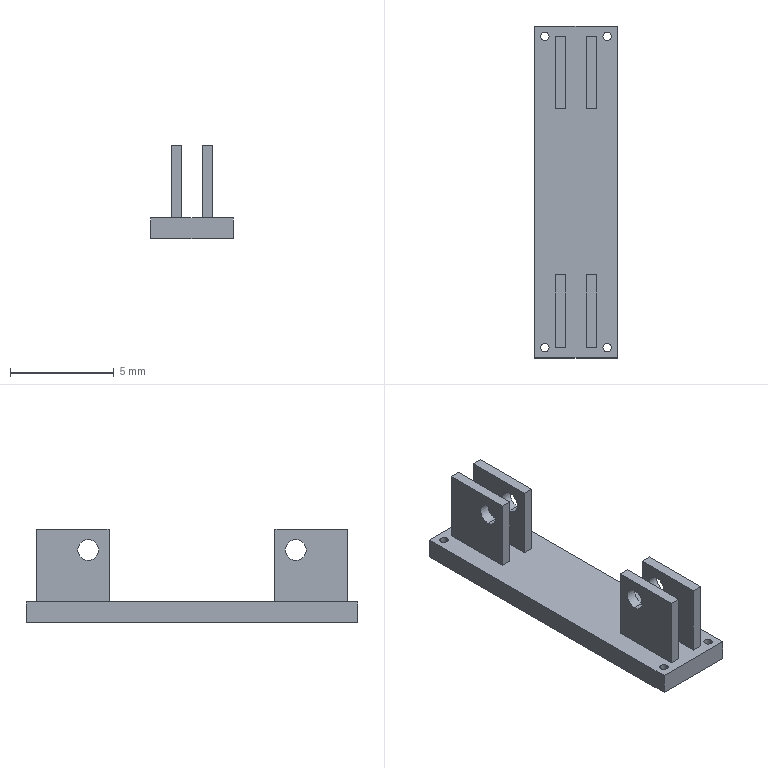Part | SolidWorks | features ICE 4, Extrusion 1 | 1 solid | 42 faces | box 4 x 16 x 4.5 mm | volume 86.427 mm3 | plane 26 | cylinder 16 | commonest cylinder face diameters 0.4 x8 1 x8
STEP:
#1=CARTESIAN_POINT('',(1.3,7.5,0.));
#2=VERTEX_POINT('',#1);
#3=CARTESIAN_POINT('',(1.7,7.5,0.));
#4=VERTEX_POINT('',#3);
#5=CARTESIAN_POINT('',(1.5,7.5,0.));
#6=DIRECTION('',(0.,0.,1.));
#7=DIRECTION('',(1.,0.,0.));
#8=AXIS2_PLACEMENT_3D('',#5,#6,#7);
#9=CIRCLE('',#8,0.2);
#10=EDGE_CURVE('',#2,#4,#9,.T.);
#11=ORIENTED_EDGE('',*,*,#10,.F.);
#12=CARTESIAN_POINT('',(1.3,7.5,1.));
#13=VERTEX_POINT('',#12);
#14=CARTESIAN_POINT('',(1.3,7.5,-3.5));
#15=DIRECTION('',(0.,0.,1.));
#16=VECTOR('',#15,1000.);
#17=LINE('',#14,#16);
#18=EDGE_CURVE('',#2,#13,#17,.T.);
#19=ORIENTED_EDGE('',*,*,#18,.T.);
#20=CARTESIAN_POINT('',(1.7,7.5,1.));
#21=VERTEX_POINT('',#20);
#22=CARTESIAN_POINT('',(1.5,7.5,1.));
#23=DIRECTION('',(0.,0.,1.));
#24=DIRECTION('',(1.,0.,0.));
#25=AXIS2_PLACEMENT_3D('',#22,#23,#24);
#26=CIRCLE('',#25,0.2);
#27=EDGE_CURVE('',#13,#21,#26,.T.);
#28=ORIENTED_EDGE('',*,*,#27,.T.);
#29=CARTESIAN_POINT('',(1.7,7.5,-3.5));
#30=DIRECTION('',(0.,0.,1.));
#31=VECTOR('',#30,1000.);
#32=LINE('',#29,#31);
#33=EDGE_CURVE('',#4,#21,#32,.T.);
#34=ORIENTED_EDGE('',*,*,#33,.F.);
#35=EDGE_LOOP('',(#11,#19,#28,#34));
#36=FACE_OUTER_BOUND('',#35,.T.);
#37=CARTESIAN_POINT('',(1.5,7.5,-3.5));
#38=DIRECTION('',(0.,0.,1.));
#39=DIRECTION('',(1.,0.,0.));
#40=AXIS2_PLACEMENT_3D('',#37,#38,#39);
#41=CYLINDRICAL_SURFACE('',#40,0.2);
#42=ADVANCED_FACE('',(#36),#41,.F.);
#43=CARTESIAN_POINT('',(1.3,-7.5,0.));
#44=VERTEX_POINT('',#43);
#45=CARTESIAN_POINT('',(1.7,-7.5,0.));
#46=VERTEX_POINT('',#45);
#47=CARTESIAN_POINT('',(1.5,-7.5,0.));
#48=DIRECTION('',(0.,0.,1.));
#49=DIRECTION('',(1.,0.,0.));
#50=AXIS2_PLACEMENT_3D('',#47,#48,#49);
#51=CIRCLE('',#50,0.2);
#52=EDGE_CURVE('',#44,#46,#51,.T.);
#53=ORIENTED_EDGE('',*,*,#52,.F.);
#54=CARTESIAN_POINT('',(1.3,-7.5,1.));
#55=VERTEX_POINT('',#54);
#56=CARTESIAN_POINT('',(1.3,-7.5,-3.5));
#57=DIRECTION('',(0.,0.,1.));
#58=VECTOR('',#57,1000.);
#59=LINE('',#56,#58);
#60=EDGE_CURVE('',#44,#55,#59,.T.);
#61=ORIENTED_EDGE('',*,*,#60,.T.);
#62=CARTESIAN_POINT('',(1.7,-7.5,1.));
#63=VERTEX_POINT('',#62);
#64=CARTESIAN_POINT('',(1.5,-7.5,1.));
#65=DIRECTION('',(0.,0.,1.));
#66=DIRECTION('',(1.,0.,0.));
#67=AXIS2_PLACEMENT_3D('',#64,#65,#66);
#68=CIRCLE('',#67,0.2);
#69=EDGE_CURVE('',#55,#63,#68,.T.);
#70=ORIENTED_EDGE('',*,*,#69,.T.);
#71=CARTESIAN_POINT('',(1.7,-7.5,-3.5));
#72=DIRECTION('',(0.,0.,1.));
#73=VECTOR('',#72,1000.);
#74=LINE('',#71,#73);
#75=EDGE_CURVE('',#46,#63,#74,.T.);
#76=ORIENTED_EDGE('',*,*,#75,.F.);
#77=EDGE_LOOP('',(#53,#61,#70,#76));
#78=FACE_OUTER_BOUND('',#77,.T.);
#79=CARTESIAN_POINT('',(1.5,-7.5,-3.5));
#80=DIRECTION('',(0.,0.,1.));
#81=DIRECTION('',(1.,0.,0.));
#82=AXIS2_PLACEMENT_3D('',#79,#80,#81);
#83=CYLINDRICAL_SURFACE('',#82,0.2);
#84=ADVANCED_FACE('',(#78),#83,.F.);
#85=CARTESIAN_POINT('',(-1.7,-7.5,0.));
#86=VERTEX_POINT('',#85);
#87=CARTESIAN_POINT('',(-1.3,-7.5,0.));
#88=VERTEX_POINT('',#87);
#89=CARTESIAN_POINT('',(-1.5,-7.5,0.));
#90=DIRECTION('',(0.,0.,1.));
#91=DIRECTION('',(1.,0.,0.));
#92=AXIS2_PLACEMENT_3D('',#89,#90,#91);
#93=CIRCLE('',#92,0.2);
#94=EDGE_CURVE('',#86,#88,#93,.T.);
#95=ORIENTED_EDGE('',*,*,#94,.F.);
#96=CARTESIAN_POINT('',(-1.7,-7.5,1.));
#97=VERTEX_POINT('',#96);
#98=CARTESIAN_POINT('',(-1.7,-7.5,-3.5));
#99=DIRECTION('',(0.,0.,1.));
#100=VECTOR('',#99,1000.);
#101=LINE('',#98,#100);
#102=EDGE_CURVE('',#86,#97,#101,.T.);
#103=ORIENTED_EDGE('',*,*,#102,.T.);
#104=CARTESIAN_POINT('',(-1.3,-7.5,1.));
#105=VERTEX_POINT('',#104);
#106=CARTESIAN_POINT('',(-1.5,-7.5,1.));
#107=DIRECTION('',(0.,0.,1.));
#108=DIRECTION('',(1.,0.,0.));
#109=AXIS2_PLACEMENT_3D('',#106,#107,#108);
#110=CIRCLE('',#109,0.2);
#111=EDGE_CURVE('',#97,#105,#110,.T.);
#112=ORIENTED_EDGE('',*,*,#111,.T.);
#113=CARTESIAN_POINT('',(-1.3,-7.5,-3.5));
#114=DIRECTION('',(0.,0.,1.));
#115=VECTOR('',#114,1000.);
#116=LINE('',#113,#115);
#117=EDGE_CURVE('',#88,#105,#116,.T.);
#118=ORIENTED_EDGE('',*,*,#117,.F.);
#119=EDGE_LOOP('',(#95,#103,#112,#118));
#120=FACE_OUTER_BOUND('',#119,.T.);
#121=CARTESIAN_POINT('',(-1.5,-7.5,-3.5));
#122=DIRECTION('',(0.,0.,1.));
#123=DIRECTION('',(1.,0.,0.));
#124=AXIS2_PLACEMENT_3D('',#121,#122,#123);
#125=CYLINDRICAL_SURFACE('',#124,0.2);
#126=ADVANCED_FACE('',(#120),#125,.F.);
#127=CARTESIAN_POINT('',(-1.7,7.5,0.));
#128=VERTEX_POINT('',#127);
#129=CARTESIAN_POINT('',(-1.3,7.5,0.));
#130=VERTEX_POINT('',#129);
#131=CARTESIAN_POINT('',(-1.5,7.5,0.));
#132=DIRECTION('',(0.,0.,1.));
#133=DIRECTION('',(1.,0.,0.));
#134=AXIS2_PLACEMENT_3D('',#131,#132,#133);
#135=CIRCLE('',#134,0.2);
#136=EDGE_CURVE('',#128,#130,#135,.T.);
#137=ORIENTED_EDGE('',*,*,#136,.F.);
#138=CARTESIAN_POINT('',(-1.7,7.5,1.));
#139=VERTEX_POINT('',#138);
#140=CARTESIAN_POINT('',(-1.7,7.5,-3.5));
#141=DIRECTION('',(0.,0.,1.));
#142=VECTOR('',#141,1000.);
#143=LINE('',#140,#142);
#144=EDGE_CURVE('',#128,#139,#143,.T.);
#145=ORIENTED_EDGE('',*,*,#144,.T.);
#146=CARTESIAN_POINT('',(-1.3,7.5,1.));
#147=VERTEX_POINT('',#146);
#148=CARTESIAN_POINT('',(-1.5,7.5,1.));
#149=DIRECTION('',(0.,0.,1.));
#150=DIRECTION('',(1.,0.,0.));
#151=AXIS2_PLACEMENT_3D('',#148,#149,#150);
#152=CIRCLE('',#151,0.2);
#153=EDGE_CURVE('',#139,#147,#152,.T.);
#154=ORIENTED_EDGE('',*,*,#153,.T.);
#155=CARTESIAN_POINT('',(-1.3,7.5,-3.5));
#156=DIRECTION('',(0.,0.,1.));
#157=VECTOR('',#156,1000.);
#158=LINE('',#155,#157);
#159=EDGE_CURVE('',#130,#147,#158,.T.);
#160=ORIENTED_EDGE('',*,*,#159,.F.);
#161=EDGE_LOOP('',(#137,#145,#154,#160));
#162=FACE_OUTER_BOUND('',#161,.T.);
#163=CARTESIAN_POINT('',(-1.5,7.5,-3.5));
#164=DIRECTION('',(0.,0.,1.));
#165=DIRECTION('',(1.,0.,0.));
#166=AXIS2_PLACEMENT_3D('',#163,#164,#165);
#167=CYLINDRICAL_SURFACE('',#166,0.2);
#168=ADVANCED_FACE('',(#162),#167,.F.);
#169=CARTESIAN_POINT('',(1.,5.,3.));
#170=VERTEX_POINT('',#169);
#171=CARTESIAN_POINT('',(1.,5.,4.));
#172=VERTEX_POINT('',#171);
#173=CARTESIAN_POINT('',(1.,5.,3.5));
#174=DIRECTION('',(-1.,0.,0.));
#175=DIRECTION('',(0.,0.,1.));
#176=AXIS2_PLACEMENT_3D('',#173,#174,#175);
#177=CIRCLE('',#176,0.5);
#178=EDGE_CURVE('',#170,#172,#177,.T.);
#179=ORIENTED_EDGE('',*,*,#178,.F.);
#180=CARTESIAN_POINT('',(0.5,5.,3.));
#181=VERTEX_POINT('',#180);
#182=CARTESIAN_POINT('',(3.5,5.,3.));
#183=DIRECTION('',(-1.,0.,0.));
#184=VECTOR('',#183,1000.);
#185=LINE('',#182,#184);
#186=EDGE_CURVE('',#170,#181,#185,.T.);
#187=ORIENTED_EDGE('',*,*,#186,.T.);
#188=CARTESIAN_POINT('',(0.5,5.,4.));
#189=VERTEX_POINT('',#188);
#190=CARTESIAN_POINT('',(0.5,5.,3.5));
#191=DIRECTION('',(1.,0.,0.));
#192=DIRECTION('',(0.,0.,-1.));
#193=AXIS2_PLACEMENT_3D('',#190,#191,#192);
#194=CIRCLE('',#193,0.5);
#195=EDGE_CURVE('',#189,#181,#194,.T.);
#196=ORIENTED_EDGE('',*,*,#195,.F.);
#197=CARTESIAN_POINT('',(3.5,5.,4.));
#198=DIRECTION('',(-1.,0.,0.));
#199=VECTOR('',#198,1000.);
#200=LINE('',#197,#199);
#201=EDGE_CURVE('',#172,#189,#200,.T.);
#202=ORIENTED_EDGE('',*,*,#201,.F.);
#203=EDGE_LOOP('',(#179,#187,#196,#202));
#204=FACE_OUTER_BOUND('',#203,.T.);
#205=CARTESIAN_POINT('',(3.5,5.,3.5));
#206=DIRECTION('',(-1.,0.,0.));
#207=DIRECTION('',(0.,0.,1.));
#208=AXIS2_PLACEMENT_3D('',#205,#206,#207);
#209=CYLINDRICAL_SURFACE('',#208,0.5);
#210=ADVANCED_FACE('',(#204),#209,.F.);
#211=CARTESIAN_POINT('',(1.,-5.,3.));
#212=VERTEX_POINT('',#211);
#213=CARTESIAN_POINT('',(1.,-5.,4.));
#214=VERTEX_POINT('',#213);
#215=CARTESIAN_POINT('',(1.,-5.,3.5));
#216=DIRECTION('',(-1.,0.,0.));
#217=DIRECTION('',(0.,0.,1.));
#218=AXIS2_PLACEMENT_3D('',#215,#216,#217);
#219=CIRCLE('',#218,0.5);
#220=EDGE_CURVE('',#212,#214,#219,.T.);
#221=ORIENTED_EDGE('',*,*,#220,.F.);
#222=CARTESIAN_POINT('',(0.5,-5.,3.));
#223=VERTEX_POINT('',#222);
#224=CARTESIAN_POINT('',(3.5,-5.,3.));
#225=DIRECTION('',(-1.,0.,0.));
#226=VECTOR('',#225,1000.);
#227=LINE('',#224,#226);
#228=EDGE_CURVE('',#212,#223,#227,.T.);
#229=ORIENTED_EDGE('',*,*,#228,.T.);
#230=CARTESIAN_POINT('',(0.5,-5.,4.));
#231=VERTEX_POINT('',#230);
#232=CARTESIAN_POINT('',(0.5,-5.,3.5));
#233=DIRECTION('',(1.,0.,0.));
#234=DIRECTION('',(0.,0.,-1.));
#235=AXIS2_PLACEMENT_3D('',#232,#233,#234);
#236=CIRCLE('',#235,0.5);
#237=EDGE_CURVE('',#231,#223,#236,.T.);
#238=ORIENTED_EDGE('',*,*,#237,.F.);
#239=CARTESIAN_POINT('',(3.5,-5.,4.));
#240=DIRECTION('',(-1.,0.,0.));
#241=VECTOR('',#240,1000.);
#242=LINE('',#239,#241);
#243=EDGE_CURVE('',#214,#231,#242,.T.);
#244=ORIENTED_EDGE('',*,*,#243,.F.);
#245=EDGE_LOOP('',(#221,#229,#238,#244));
#246=FACE_OUTER_BOUND('',#245,.T.);
#247=CARTESIAN_POINT('',(3.5,-5.,3.5));
#248=DIRECTION('',(-1.,0.,0.));
#249=DIRECTION('',(0.,0.,1.));
#250=AXIS2_PLACEMENT_3D('',#247,#248,#249);
#251=CYLINDRICAL_SURFACE('',#250,0.5);
#252=ADVANCED_FACE('',(#246),#251,.F.);
#253=CARTESIAN_POINT('',(-0.5,5.,3.));
#254=VERTEX_POINT('',#253);
#255=CARTESIAN_POINT('',(-0.5,5.,4.));
#256=VERTEX_POINT('',#255);
#257=CARTESIAN_POINT('',(-0.5,5.,3.5));
#258=DIRECTION('',(-1.,0.,0.));
#259=DIRECTION('',(0.,0.,1.));
#260=AXIS2_PLACEMENT_3D('',#257,#258,#259);
#261=CIRCLE('',#260,0.5);
#262=EDGE_CURVE('',#254,#256,#261,.T.);
#263=ORIENTED_EDGE('',*,*,#262,.F.);
#264=CARTESIAN_POINT('',(-1.,5.,3.));
#265=VERTEX_POINT('',#264);
#266=CARTESIAN_POINT('',(3.5,5.,3.));
#267=DIRECTION('',(-1.,0.,0.));
#268=VECTOR('',#267,1000.);
#269=LINE('',#266,#268);
#270=EDGE_CURVE('',#254,#265,#269,.T.);
#271=ORIENTED_EDGE('',*,*,#270,.T.);
#272=CARTESIAN_POINT('',(-1.,5.,4.));
#273=VERTEX_POINT('',#272);
#274=CARTESIAN_POINT('',(-1.,5.,3.5));
#275=DIRECTION('',(-1.,0.,0.));
#276=DIRECTION('',(0.,0.,1.));
#277=AXIS2_PLACEMENT_3D('',#274,#275,#276);
#278=CIRCLE('',#277,0.5);
#279=EDGE_CURVE('',#265,#273,#278,.T.);
#280=ORIENTED_EDGE('',*,*,#279,.T.);
#281=CARTESIAN_POINT('',(3.5,5.,4.));
#282=DIRECTION('',(-1.,0.,0.));
#283=VECTOR('',#282,1000.);
#284=LINE('',#281,#283);
#285=EDGE_CURVE('',#256,#273,#284,.T.);
#286=ORIENTED_EDGE('',*,*,#285,.F.);
#287=EDGE_LOOP('',(#263,#271,#280,#286));
#288=FACE_OUTER_BOUND('',#287,.T.);
#289=CARTESIAN_POINT('',(3.5,5.,3.5));
#290=DIRECTION('',(-1.,0.,0.));
#291=DIRECTION('',(0.,0.,1.));
#292=AXIS2_PLACEMENT_3D('',#289,#290,#291);
#293=CYLINDRICAL_SURFACE('',#292,0.5);
#294=ADVANCED_FACE('',(#288),#293,.F.);
#295=CARTESIAN_POINT('',(-0.5,-5.,3.));
#296=VERTEX_POINT('',#295);
#297=CARTESIAN_POINT('',(-0.5,-5.,4.));
#298=VERTEX_POINT('',#297);
#299=CARTESIAN_POINT('',(-0.5,-5.,3.5));
#300=DIRECTION('',(-1.,0.,0.));
#301=DIRECTION('',(0.,0.,1.));
#302=AXIS2_PLACEMENT_3D('',#299,#300,#301);
#303=CIRCLE('',#302,0.5);
#304=EDGE_CURVE('',#296,#298,#303,.T.);
#305=ORIENTED_EDGE('',*,*,#304,.F.);
#306=CARTESIAN_POINT('',(-1.,-5.,3.));
#307=VERTEX_POINT('',#306);
#308=CARTESIAN_POINT('',(3.5,-5.,3.));
#309=DIRECTION('',(-1.,0.,0.));
#310=VECTOR('',#309,1000.);
#311=LINE('',#308,#310);
#312=EDGE_CURVE('',#296,#307,#311,.T.);
#313=ORIENTED_EDGE('',*,*,#312,.T.);
#314=CARTESIAN_POINT('',(-1.,-5.,4.));
#315=VERTEX_POINT('',#314);
#316=CARTESIAN_POINT('',(-1.,-5.,3.5));
#317=DIRECTION('',(-1.,0.,0.));
#318=DIRECTION('',(0.,0.,1.));
#319=AXIS2_PLACEMENT_3D('',#316,#317,#318);
#320=CIRCLE('',#319,0.5);
#321=EDGE_CURVE('',#307,#315,#320,.T.);
#322=ORIENTED_EDGE('',*,*,#321,.T.);
#323=CARTESIAN_POINT('',(3.5,-5.,4.));
#324=DIRECTION('',(-1.,0.,0.));
#325=VECTOR('',#324,1000.);
#326=LINE('',#323,#325);
#327=EDGE_CURVE('',#298,#315,#326,.T.);
#328=ORIENTED_EDGE('',*,*,#327,.F.);
#329=EDGE_LOOP('',(#305,#313,#322,#328));
#330=FACE_OUTER_BOUND('',#329,.T.);
#331=CARTESIAN_POINT('',(3.5,-5.,3.5));
#332=DIRECTION('',(-1.,0.,0.));
#333=DIRECTION('',(0.,0.,1.));
#334=AXIS2_PLACEMENT_3D('',#331,#332,#333);
#335=CYLINDRICAL_SURFACE('',#334,0.5);
#336=ADVANCED_FACE('',(#330),#335,.F.);
#337=CARTESIAN_POINT('',(1.,-5.,3.5));
#338=DIRECTION('',(-1.,0.,0.));
#339=DIRECTION('',(0.,0.,1.));
#340=AXIS2_PLACEMENT_3D('',#337,#338,#339);
#341=CIRCLE('',#340,0.5);
#342=EDGE_CURVE('',#214,#212,#341,.T.);
#343=ORIENTED_EDGE('',*,*,#342,.T.);
#344=ORIENTED_EDGE('',*,*,#220,.T.);
#345=EDGE_LOOP('',(#343,#344));
#346=FACE_BOUND('',#345,.T.);
#347=CARTESIAN_POINT('',(1.,-7.5,1.));
#348=VERTEX_POINT('',#347);
#349=CARTESIAN_POINT('',(1.,-4.,1.));
#350=VERTEX_POINT('',#349);
#351=CARTESIAN_POINT('',(1.,-7.5,1.));
#352=DIRECTION('',(0.,1.,0.));
#353=VECTOR('',#352,1000.);
#354=LINE('',#351,#353);
#355=EDGE_CURVE('',#348,#350,#354,.T.);
#356=ORIENTED_EDGE('',*,*,#355,.T.);
#357=CARTESIAN_POINT('',(1.,-4.,4.5));
#358=VERTEX_POINT('',#357);
#359=CARTESIAN_POINT('',(1.,-4.,4.5));
#360=DIRECTION('',(0.,0.,1.));
#361=VECTOR('',#360,1000.);
#362=LINE('',#359,#361);
#363=EDGE_CURVE('',#350,#358,#362,.T.);
#364=ORIENTED_EDGE('',*,*,#363,.T.);
#365=CARTESIAN_POINT('',(1.,-7.5,4.5));
#366=VERTEX_POINT('',#365);
#367=CARTESIAN_POINT('',(1.,-7.5,4.5));
#368=DIRECTION('',(0.,1.,0.));
#369=VECTOR('',#368,1000.);
#370=LINE('',#367,#369);
#371=EDGE_CURVE('',#366,#358,#370,.T.);
#372=ORIENTED_EDGE('',*,*,#371,.F.);
#373=CARTESIAN_POINT('',(1.,-7.5,4.5));
#374=DIRECTION('',(0.,0.,-1.));
#375=VECTOR('',#374,1000.);
#376=LINE('',#373,#375);
#377=EDGE_CURVE('',#366,#348,#376,.T.);
#378=ORIENTED_EDGE('',*,*,#377,.T.);
#379=EDGE_LOOP('',(#356,#364,#372,#378));
#380=FACE_OUTER_BOUND('',#379,.T.);
#381=CARTESIAN_POINT('',(1.,-7.5,4.5));
#382=DIRECTION('',(-1.,0.,0.));
#383=DIRECTION('',(0.,0.,1.));
#384=AXIS2_PLACEMENT_3D('',#381,#382,#383);
#385=PLANE('',#384);
#386=ADVANCED_FACE('',(#346,#380),#385,.F.);
#387=ORIENTED_EDGE('',*,*,#237,.T.);
#388=CARTESIAN_POINT('',(0.5,-5.,3.5));
#389=DIRECTION('',(1.,0.,0.));
#390=DIRECTION('',(0.,0.,-1.));
#391=AXIS2_PLACEMENT_3D('',#388,#389,#390);
#392=CIRCLE('',#391,0.5);
#393=EDGE_CURVE('',#223,#231,#392,.T.);
#394=ORIENTED_EDGE('',*,*,#393,.T.);
#395=EDGE_LOOP('',(#387,#394));
#396=FACE_BOUND('',#395,.T.);
#397=CARTESIAN_POINT('',(0.5,-4.,4.5));
#398=VERTEX_POINT('',#397);
#399=CARTESIAN_POINT('',(0.5,-7.5,4.5));
#400=VERTEX_POINT('',#399);
#401=CARTESIAN_POINT('',(0.5,-7.5,4.5));
#402=DIRECTION('',(0.,-1.,0.));
#403=VECTOR('',#402,1000.);
#404=LINE('',#401,#403);
#405=EDGE_CURVE('',#398,#400,#404,.T.);
#406=ORIENTED_EDGE('',*,*,#405,.F.);
#407=CARTESIAN_POINT('',(0.5,-4.,1.));
#408=VERTEX_POINT('',#407);
#409=CARTESIAN_POINT('',(0.5,-4.,4.5));
#410=DIRECTION('',(0.,0.,-1.));
#411=VECTOR('',#410,1000.);
#412=LINE('',#409,#411);
#413=EDGE_CURVE('',#398,#408,#412,.T.);
#414=ORIENTED_EDGE('',*,*,#413,.T.);
#415=CARTESIAN_POINT('',(0.5,-7.5,1.));
#416=VERTEX_POINT('',#415);
#417=CARTESIAN_POINT('',(0.5,-7.5,1.));
#418=DIRECTION('',(0.,-1.,0.));
#419=VECTOR('',#418,1000.);
#420=LINE('',#417,#419);
#421=EDGE_CURVE('',#408,#416,#420,.T.);
#422=ORIENTED_EDGE('',*,*,#421,.T.);
#423=CARTESIAN_POINT('',(0.5,-7.5,4.5));
#424=DIRECTION('',(0.,0.,-1.));
#425=VECTOR('',#424,1000.);
#426=LINE('',#423,#425);
#427=EDGE_CURVE('',#400,#416,#426,.T.);
#428=ORIENTED_EDGE('',*,*,#427,.F.);
#429=EDGE_LOOP('',(#406,#414,#422,#428));
#430=FACE_OUTER_BOUND('',#429,.T.);
#431=CARTESIAN_POINT('',(0.5,-7.5,4.5));
#432=DIRECTION('',(1.,0.,0.));
#433=DIRECTION('',(0.,0.,-1.));
#434=AXIS2_PLACEMENT_3D('',#431,#432,#433);
#435=PLANE('',#434);
#436=ADVANCED_FACE('',(#396,#430),#435,.F.);
#437=ORIENTED_EDGE('',*,*,#371,.T.);
#438=CARTESIAN_POINT('',(-4.096,-4.,4.5));
#439=DIRECTION('',(1.,0.,0.));
#440=VECTOR('',#439,1000.);
#441=LINE('',#438,#440);
#442=EDGE_CURVE('',#398,#358,#441,.T.);
#443=ORIENTED_EDGE('',*,*,#442,.F.);
#444=ORIENTED_EDGE('',*,*,#405,.T.);
#445=CARTESIAN_POINT('',(0.5,-7.5,4.5));
#446=DIRECTION('',(1.,0.,0.));
#447=VECTOR('',#446,1000.);
#448=LINE('',#445,#447);
#449=EDGE_CURVE('',#400,#366,#448,.T.);
#450=ORIENTED_EDGE('',*,*,#449,.T.);
#451=EDGE_LOOP('',(#437,#443,#444,#450));
#452=FACE_OUTER_BOUND('',#451,.T.);
#453=CARTESIAN_POINT('',(0.,0.,4.5));
#454=DIRECTION('',(0.,0.,-1.));
#455=DIRECTION('',(-1.,0.,0.));
#456=AXIS2_PLACEMENT_3D('',#453,#454,#455);
#457=PLANE('',#456);
#458=ADVANCED_FACE('',(#452),#457,.F.);
#459=CARTESIAN_POINT('',(-1.,-5.,3.5));
#460=DIRECTION('',(-1.,0.,0.));
#461=DIRECTION('',(0.,0.,1.));
#462=AXIS2_PLACEMENT_3D('',#459,#460,#461);
#463=CIRCLE('',#462,0.5);
#464=EDGE_CURVE('',#315,#307,#463,.T.);
#465=ORIENTED_EDGE('',*,*,#464,.F.);
#466=ORIENTED_EDGE('',*,*,#321,.F.);
#467=EDGE_LOOP('',(#465,#466));
#468=FACE_BOUND('',#467,.T.);
#469=CARTESIAN_POINT('',(-1.,-4.,4.5));
#470=VERTEX_POINT('',#469);
#471=CARTESIAN_POINT('',(-1.,-7.5,4.5));
#472=VERTEX_POINT('',#471);
#473=CARTESIAN_POINT('',(-1.,-7.5,4.5));
#474=DIRECTION('',(0.,-1.,0.));
#475=VECTOR('',#474,1000.);
#476=LINE('',#473,#475);
#477=EDGE_CURVE('',#470,#472,#476,.T.);
#478=ORIENTED_EDGE('',*,*,#477,.F.);
#479=CARTESIAN_POINT('',(-1.,-4.,1.));
#480=VERTEX_POINT('',#479);
#481=CARTESIAN_POINT('',(-1.,-4.,4.5));
#482=DIRECTION('',(0.,0.,-1.));
#483=VECTOR('',#482,1000.);
#484=LINE('',#481,#483);
#485=EDGE_CURVE('',#470,#480,#484,.T.);
#486=ORIENTED_EDGE('',*,*,#485,.T.);
#487=CARTESIAN_POINT('',(-1.,-7.5,1.));
#488=VERTEX_POINT('',#487);
#489=CARTESIAN_POINT('',(-1.,-7.5,1.));
#490=DIRECTION('',(0.,-1.,0.));
#491=VECTOR('',#490,1000.);
#492=LINE('',#489,#491);
#493=EDGE_CURVE('',#480,#488,#492,.T.);
#494=ORIENTED_EDGE('',*,*,#493,.T.);
#495=CARTESIAN_POINT('',(-1.,-7.5,4.5));
#496=DIRECTION('',(0.,0.,-1.));
#497=VECTOR('',#496,1000.);
#498=LINE('',#495,#497);
#499=EDGE_CURVE('',#472,#488,#498,.T.);
#500=ORIENTED_EDGE('',*,*,#499,.F.);
#501=EDGE_LOOP('',(#478,#486,#494,#500));
#502=FACE_OUTER_BOUND('',#501,.T.);
#503=CARTESIAN_POINT('',(-1.,-7.5,4.5));
#504=DIRECTION('',(1.,0.,0.));
#505=DIRECTION('',(0.,1.,0.));
#506=AXIS2_PLACEMENT_3D('',#503,#504,#505);
#507=PLANE('',#506);
#508=ADVANCED_FACE('',(#468,#502),#507,.F.);
#509=CARTESIAN_POINT('',(-0.5,-5.,3.5));
#510=DIRECTION('',(-1.,0.,0.));
#511=DIRECTION('',(0.,0.,1.));
#512=AXIS2_PLACEMENT_3D('',#509,#510,#511);
#513=CIRCLE('',#512,0.5);
#514=EDGE_CURVE('',#298,#296,#513,.T.);
#515=ORIENTED_EDGE('',*,*,#514,.T.);
#516=ORIENTED_EDGE('',*,*,#304,.T.);
#517=EDGE_LOOP('',(#515,#516));
#518=FACE_BOUND('',#517,.T.);
#519=CARTESIAN_POINT('',(-0.5,-7.5,1.));
#520=VERTEX_POINT('',#519);
#521=CARTESIAN_POINT('',(-0.5,-4.,1.));
#522=VERTEX_POINT('',#521);
#523=CARTESIAN_POINT('',(-0.5,-7.5,1.));
#524=DIRECTION('',(0.,1.,0.));
#525=VECTOR('',#524,1000.);
#526=LINE('',#523,#525);
#527=EDGE_CURVE('',#520,#522,#526,.T.);
#528=ORIENTED_EDGE('',*,*,#527,.T.);
#529=CARTESIAN_POINT('',(-0.5,-4.,4.5));
#530=VERTEX_POINT('',#529);
#531=CARTESIAN_POINT('',(-0.5,-4.,4.5));
#532=DIRECTION('',(0.,0.,1.));
#533=VECTOR('',#532,1000.);
#534=LINE('',#531,#533);
#535=EDGE_CURVE('',#522,#530,#534,.T.);
#536=ORIENTED_EDGE('',*,*,#535,.T.);
#537=CARTESIAN_POINT('',(-0.5,-7.5,4.5));
#538=VERTEX_POINT('',#537);
#539=CARTESIAN_POINT('',(-0.5,-7.5,4.5));
#540=DIRECTION('',(0.,1.,0.));
#541=VECTOR('',#540,1000.);
#542=LINE('',#539,#541);
#543=EDGE_CURVE('',#538,#530,#542,.T.);
#544=ORIENTED_EDGE('',*,*,#543,.F.);
#545=CARTESIAN_POINT('',(-0.5,-7.5,4.5));
#546=DIRECTION('',(0.,0.,-1.));
#547=VECTOR('',#546,1000.);
#548=LINE('',#545,#547);
#549=EDGE_CURVE('',#538,#520,#548,.T.);
#550=ORIENTED_EDGE('',*,*,#549,.T.);
#551=EDGE_LOOP('',(#528,#536,#544,#550));
#552=FACE_OUTER_BOUND('',#551,.T.);
#553=CARTESIAN_POINT('',(-0.5,-7.5,4.5));
#554=DIRECTION('',(-1.,0.,0.));
#555=DIRECTION('',(0.,0.,1.));
#556=AXIS2_PLACEMENT_3D('',#553,#554,#555);
#557=PLANE('',#556);
#558=ADVANCED_FACE('',(#518,#552),#557,.F.);
#559=CARTESIAN_POINT('',(0.,-4.,4.5));
#560=DIRECTION('',(1.,0.,0.));
#561=VECTOR('',#560,1000.);
#562=LINE('',#559,#561);
#563=EDGE_CURVE('',#470,#530,#562,.T.);
#564=ORIENTED_EDGE('',*,*,#563,.F.);
#565=ORIENTED_EDGE('',*,*,#477,.T.);
#566=CARTESIAN_POINT('',(-0.5,-7.5,4.5));
#567=DIRECTION('',(1.,0.,0.));
#568=VECTOR('',#567,1000.);
#569=LINE('',#566,#568);
#570=EDGE_CURVE('',#472,#538,#569,.T.);
#571=ORIENTED_EDGE('',*,*,#570,.T.);
#572=ORIENTED_EDGE('',*,*,#543,.T.);
#573=EDGE_LOOP('',(#564,#565,#571,#572));
#574=FACE_OUTER_BOUND('',#573,.T.);
#575=CARTESIAN_POINT('',(0.,0.,4.5));
#576=DIRECTION('',(0.,0.,1.));
#577=DIRECTION('',(1.,0.,0.));
#578=AXIS2_PLACEMENT_3D('',#575,#576,#577);
#579=PLANE('',#578);
#580=ADVANCED_FACE('',(#574),#579,.T.);
#581=ORIENTED_EDGE('',*,*,#493,.F.);
#582=CARTESIAN_POINT('',(-4.096,-4.,1.));
#583=DIRECTION('',(-1.,0.,0.));
#584=VECTOR('',#583,1000.);
#585=LINE('',#582,#584);
#586=EDGE_CURVE('',#522,#480,#585,.T.);
#587=ORIENTED_EDGE('',*,*,#586,.F.);
#588=ORIENTED_EDGE('',*,*,#527,.F.);
#589=CARTESIAN_POINT('',(-0.5,-7.5,1.));
#590=DIRECTION('',(1.,0.,0.));
#591=VECTOR('',#590,1000.);
#592=LINE('',#589,#591);
#593=EDGE_CURVE('',#488,#520,#592,.T.);
#594=ORIENTED_EDGE('',*,*,#593,.F.);
#595=EDGE_LOOP('',(#581,#587,#588,#594));
#596=FACE_BOUND('',#595,.T.);
#597=ORIENTED_EDGE('',*,*,#421,.F.);
#598=CARTESIAN_POINT('',(-4.096,-4.,1.));
#599=DIRECTION('',(-1.,0.,0.));
#600=VECTOR('',#599,1000.);
#601=LINE('',#598,#600);
#602=EDGE_CURVE('',#350,#408,#601,.T.);
#603=ORIENTED_EDGE('',*,*,#602,.F.);
#604=ORIENTED_EDGE('',*,*,#355,.F.);
#605=CARTESIAN_POINT('',(0.5,-7.5,1.));
#606=DIRECTION('',(1.,0.,0.));
#607=VECTOR('',#606,1000.);
#608=LINE('',#605,#607);
#609=EDGE_CURVE('',#416,#348,#608,.T.);
#610=ORIENTED_EDGE('',*,*,#609,.F.);
#611=EDGE_LOOP('',(#597,#603,#604,#610));
#612=FACE_BOUND('',#611,.T.);
#613=CARTESIAN_POINT('',(1.,4.,1.));
#614=VERTEX_POINT('',#613);
#615=CARTESIAN_POINT('',(1.,7.5,1.));
#616=VERTEX_POINT('',#615);
#617=CARTESIAN_POINT('',(1.,-7.5,1.));
#618=DIRECTION('',(0.,1.,0.));
#619=VECTOR('',#618,1000.);
#620=LINE('',#617,#619);
#621=EDGE_CURVE('',#614,#616,#620,.T.);
#622=ORIENTED_EDGE('',*,*,#621,.F.);
#623=CARTESIAN_POINT('',(0.5,4.,1.));
#624=VERTEX_POINT('',#623);
#625=CARTESIAN_POINT('',(-4.096,4.,1.));
#626=DIRECTION('',(1.,0.,0.));
#627=VECTOR('',#626,1000.);
#628=LINE('',#625,#627);
#629=EDGE_CURVE('',#624,#614,#628,.T.);
#630=ORIENTED_EDGE('',*,*,#629,.F.);
#631=CARTESIAN_POINT('',(0.5,7.5,1.));
#632=VERTEX_POINT('',#631);
#633=CARTESIAN_POINT('',(0.5,-7.5,1.));
#634=DIRECTION('',(0.,-1.,0.));
#635=VECTOR('',#634,1000.);
#636=LINE('',#633,#635);
#637=EDGE_CURVE('',#632,#624,#636,.T.);
#638=ORIENTED_EDGE('',*,*,#637,.F.);
#639=CARTESIAN_POINT('',(0.5,7.5,1.));
#640=DIRECTION('',(-1.,0.,0.));
#641=VECTOR('',#640,1000.);
#642=LINE('',#639,#641);
#643=EDGE_CURVE('',#616,#632,#642,.T.);
#644=ORIENTED_EDGE('',*,*,#643,.F.);
#645=EDGE_LOOP('',(#622,#630,#638,#644));
#646=FACE_BOUND('',#645,.T.);
#647=CARTESIAN_POINT('',(-0.5,4.,1.));
#648=VERTEX_POINT('',#647);
#649=CARTESIAN_POINT('',(-0.5,7.5,1.));
#650=VERTEX_POINT('',#649);
#651=CARTESIAN_POINT('',(-0.5,-7.5,1.));
#652=DIRECTION('',(0.,1.,0.));
#653=VECTOR('',#652,1000.);
#654=LINE('',#651,#653);
#655=EDGE_CURVE('',#648,#650,#654,.T.);
#656=ORIENTED_EDGE('',*,*,#655,.F.);
#657=CARTESIAN_POINT('',(-1.,4.,1.));
#658=VERTEX_POINT('',#657);
#659=CARTESIAN_POINT('',(-4.096,4.,1.));
#660=DIRECTION('',(1.,0.,0.));
#661=VECTOR('',#660,1000.);
#662=LINE('',#659,#661);
#663=EDGE_CURVE('',#658,#648,#662,.T.);
#664=ORIENTED_EDGE('',*,*,#663,.F.);
#665=CARTESIAN_POINT('',(-1.,7.5,1.));
#666=VERTEX_POINT('',#665);
#667=CARTESIAN_POINT('',(-1.,-7.5,1.));
#668=DIRECTION('',(0.,-1.,0.));
#669=VECTOR('',#668,1000.);
#670=LINE('',#667,#669);
#671=EDGE_CURVE('',#666,#658,#670,.T.);
#672=ORIENTED_EDGE('',*,*,#671,.F.);
#673=CARTESIAN_POINT('',(-0.5,7.5,1.));
#674=DIRECTION('',(-1.,0.,0.));
#675=VECTOR('',#674,1000.);
#676=LINE('',#673,#675);
#677=EDGE_CURVE('',#650,#666,#676,.T.);
#678=ORIENTED_EDGE('',*,*,#677,.F.);
#679=EDGE_LOOP('',(#656,#664,#672,#678));
#680=FACE_BOUND('',#679,.T.);
#681=CARTESIAN_POINT('',(2.,-8.,1.));
#682=VERTEX_POINT('',#681);
#683=CARTESIAN_POINT('',(2.,8.,1.));
#684=VERTEX_POINT('',#683);
#685=CARTESIAN_POINT('',(2.,-8.,1.));
#686=DIRECTION('',(0.,1.,0.));
#687=VECTOR('',#686,1000.);
#688=LINE('',#685,#687);
#689=EDGE_CURVE('',#682,#684,#688,.T.);
#690=ORIENTED_EDGE('',*,*,#689,.T.);
#691=CARTESIAN_POINT('',(-2.,8.,1.));
#692=VERTEX_POINT('',#691);
#693=CARTESIAN_POINT('',(2.,8.,1.));
#694=DIRECTION('',(-1.,0.,0.));
#695=VECTOR('',#694,1000.);
#696=LINE('',#693,#695);
#697=EDGE_CURVE('',#684,#692,#696,.T.);
#698=ORIENTED_EDGE('',*,*,#697,.T.);
#699=CARTESIAN_POINT('',(-2.,-8.,1.));
#700=VERTEX_POINT('',#699);
#701=CARTESIAN_POINT('',(-2.,-8.,1.));
#702=DIRECTION('',(0.,-1.,0.));
#703=VECTOR('',#702,1000.);
#704=LINE('',#701,#703);
#705=EDGE_CURVE('',#692,#700,#704,.T.);
#706=ORIENTED_EDGE('',*,*,#705,.T.);
#707=CARTESIAN_POINT('',(2.,-8.,1.));
#708=DIRECTION('',(1.,0.,0.));
#709=VECTOR('',#708,1000.);
#710=LINE('',#707,#709);
#711=EDGE_CURVE('',#700,#682,#710,.T.);
#712=ORIENTED_EDGE('',*,*,#711,.T.);
#713=EDGE_LOOP('',(#690,#698,#706,#712));
#714=FACE_OUTER_BOUND('',#713,.T.);
#715=CARTESIAN_POINT('',(1.5,7.5,1.));
#716=DIRECTION('',(0.,0.,1.));
#717=DIRECTION('',(1.,0.,0.));
#718=AXIS2_PLACEMENT_3D('',#715,#716,#717);
#719=CIRCLE('',#718,0.2);
#720=EDGE_CURVE('',#21,#13,#719,.T.);
#721=ORIENTED_EDGE('',*,*,#720,.F.);
#722=ORIENTED_EDGE('',*,*,#27,.F.);
#723=EDGE_LOOP('',(#721,#722));
#724=FACE_BOUND('',#723,.T.);
#725=CARTESIAN_POINT('',(-1.5,7.5,1.));
#726=DIRECTION('',(0.,0.,1.));
#727=DIRECTION('',(1.,0.,0.));
#728=AXIS2_PLACEMENT_3D('',#725,#726,#727);
#729=CIRCLE('',#728,0.2);
#730=EDGE_CURVE('',#147,#139,#729,.T.);
#731=ORIENTED_EDGE('',*,*,#730,.F.);
#732=ORIENTED_EDGE('',*,*,#153,.F.);
#733=EDGE_LOOP('',(#731,#732));
#734=FACE_BOUND('',#733,.T.);
#735=CARTESIAN_POINT('',(-1.5,-7.5,1.));
#736=DIRECTION('',(0.,0.,1.));
#737=DIRECTION('',(1.,0.,0.));
#738=AXIS2_PLACEMENT_3D('',#735,#736,#737);
#739=CIRCLE('',#738,0.2);
#740=EDGE_CURVE('',#105,#97,#739,.T.);
#741=ORIENTED_EDGE('',*,*,#740,.F.);
#742=ORIENTED_EDGE('',*,*,#111,.F.);
#743=EDGE_LOOP('',(#741,#742));
#744=FACE_BOUND('',#743,.T.);
#745=CARTESIAN_POINT('',(1.5,-7.5,1.));
#746=DIRECTION('',(0.,0.,1.));
#747=DIRECTION('',(1.,0.,0.));
#748=AXIS2_PLACEMENT_3D('',#745,#746,#747);
#749=CIRCLE('',#748,0.2);
#750=EDGE_CURVE('',#63,#55,#749,.T.);
#751=ORIENTED_EDGE('',*,*,#750,.F.);
#752=ORIENTED_EDGE('',*,*,#69,.F.);
#753=EDGE_LOOP('',(#751,#752));
#754=FACE_BOUND('',#753,.T.);
#755=CARTESIAN_POINT('',(0.,0.,1.));
#756=DIRECTION('',(0.,0.,1.));
#757=DIRECTION('',(1.,0.,0.));
#758=AXIS2_PLACEMENT_3D('',#755,#756,#757);
#759=PLANE('',#758);
#760=ADVANCED_FACE('',(#596,#612,#646,#680,#714,#724,#734,#744,#754),#759,.T.);
#761=CARTESIAN_POINT('',(-2.,8.,0.));
#762=VERTEX_POINT('',#761);
#763=CARTESIAN_POINT('',(-2.,-8.,0.));
#764=VERTEX_POINT('',#763);
#765=CARTESIAN_POINT('',(-2.,-8.,0.));
#766=DIRECTION('',(0.,-1.,0.));
#767=VECTOR('',#766,1000.);
#768=LINE('',#765,#767);
#769=EDGE_CURVE('',#762,#764,#768,.T.);
#770=ORIENTED_EDGE('',*,*,#769,.T.);
#771=CARTESIAN_POINT('',(-2.,-8.,1.));
#772=DIRECTION('',(0.,0.,-1.));
#773=VECTOR('',#772,1000.);
#774=LINE('',#771,#773);
#775=EDGE_CURVE('',#700,#764,#774,.T.);
#776=ORIENTED_EDGE('',*,*,#775,.F.);
#777=ORIENTED_EDGE('',*,*,#705,.F.);
#778=CARTESIAN_POINT('',(-2.,8.,1.));
#779=DIRECTION('',(0.,0.,-1.));
#780=VECTOR('',#779,1000.);
#781=LINE('',#778,#780);
#782=EDGE_CURVE('',#692,#762,#781,.T.);
#783=ORIENTED_EDGE('',*,*,#782,.T.);
#784=EDGE_LOOP('',(#770,#776,#777,#783));
#785=FACE_OUTER_BOUND('',#784,.T.);
#786=CARTESIAN_POINT('',(-2.,-8.,1.));
#787=DIRECTION('',(1.,0.,0.));
#788=DIRECTION('',(0.,0.,-1.));
#789=AXIS2_PLACEMENT_3D('',#786,#787,#788);
#790=PLANE('',#789);
#791=ADVANCED_FACE('',(#785),#790,.F.);
#792=CARTESIAN_POINT('',(2.,-8.,0.));
#793=VERTEX_POINT('',#792);
#794=CARTESIAN_POINT('',(2.,-8.,0.));
#795=DIRECTION('',(1.,0.,0.));
#796=VECTOR('',#795,1000.);
#797=LINE('',#794,#796);
#798=EDGE_CURVE('',#764,#793,#797,.T.);
#799=ORIENTED_EDGE('',*,*,#798,.T.);
#800=CARTESIAN_POINT('',(2.,-8.,1.));
#801=DIRECTION('',(0.,0.,-1.));
#802=VECTOR('',#801,1000.);
#803=LINE('',#800,#802);
#804=EDGE_CURVE('',#682,#793,#803,.T.);
#805=ORIENTED_EDGE('',*,*,#804,.F.);
#806=ORIENTED_EDGE('',*,*,#711,.F.);
#807=ORIENTED_EDGE('',*,*,#775,.T.);
#808=EDGE_LOOP('',(#799,#805,#806,#807));
#809=FACE_OUTER_BOUND('',#808,.T.);
#810=CARTESIAN_POINT('',(2.,-8.,1.));
#811=DIRECTION('',(0.,1.,0.));
#812=DIRECTION('',(0.,0.,1.));
#813=AXIS2_PLACEMENT_3D('',#810,#811,#812);
#814=PLANE('',#813);
#815=ADVANCED_FACE('',(#809),#814,.F.);
#816=CARTESIAN_POINT('',(2.,8.,0.));
#817=VERTEX_POINT('',#816);
#818=CARTESIAN_POINT('',(2.,-8.,0.));
#819=DIRECTION('',(0.,1.,0.));
#820=VECTOR('',#819,1000.);
#821=LINE('',#818,#820);
#822=EDGE_CURVE('',#793,#817,#821,.T.);
#823=ORIENTED_EDGE('',*,*,#822,.T.);
#824=CARTESIAN_POINT('',(2.,8.,1.));
#825=DIRECTION('',(0.,0.,-1.));
#826=VECTOR('',#825,1000.);
#827=LINE('',#824,#826);
#828=EDGE_CURVE('',#684,#817,#827,.T.);
#829=ORIENTED_EDGE('',*,*,#828,.F.);
#830=ORIENTED_EDGE('',*,*,#689,.F.);
#831=ORIENTED_EDGE('',*,*,#804,.T.);
#832=EDGE_LOOP('',(#823,#829,#830,#831));
#833=FACE_OUTER_BOUND('',#832,.T.);
#834=CARTESIAN_POINT('',(2.,-8.,1.));
#835=DIRECTION('',(-1.,0.,0.));
#836=DIRECTION('',(0.,0.,1.));
#837=AXIS2_PLACEMENT_3D('',#834,#835,#836);
#838=PLANE('',#837);
#839=ADVANCED_FACE('',(#833),#838,.F.);
#840=CARTESIAN_POINT('',(2.,8.,0.));
#841=DIRECTION('',(-1.,0.,0.));
#842=VECTOR('',#841,1000.);
#843=LINE('',#840,#842);
#844=EDGE_CURVE('',#817,#762,#843,.T.);
#845=ORIENTED_EDGE('',*,*,#844,.T.);
#846=ORIENTED_EDGE('',*,*,#782,.F.);
#847=ORIENTED_EDGE('',*,*,#697,.F.);
#848=ORIENTED_EDGE('',*,*,#828,.T.);
#849=EDGE_LOOP('',(#845,#846,#847,#848));
#850=FACE_OUTER_BOUND('',#849,.T.);
#851=CARTESIAN_POINT('',(2.,8.,1.));
#852=DIRECTION('',(0.,-1.,0.));
#853=DIRECTION('',(1.,0.,0.));
#854=AXIS2_PLACEMENT_3D('',#851,#852,#853);
#855=PLANE('',#854);
#856=ADVANCED_FACE('',(#850),#855,.F.);
#857=CARTESIAN_POINT('',(1.5,7.5,0.));
#858=DIRECTION('',(0.,0.,1.));
#859=DIRECTION('',(1.,0.,0.));
#860=AXIS2_PLACEMENT_3D('',#857,#858,#859);
#861=CIRCLE('',#860,0.2);
#862=EDGE_CURVE('',#4,#2,#861,.T.);
#863=ORIENTED_EDGE('',*,*,#862,.T.);
#864=ORIENTED_EDGE('',*,*,#10,.T.);
#865=EDGE_LOOP('',(#863,#864));
#866=FACE_BOUND('',#865,.T.);
#867=CARTESIAN_POINT('',(1.5,-7.5,0.));
#868=DIRECTION('',(0.,0.,1.));
#869=DIRECTION('',(1.,0.,0.));
#870=AXIS2_PLACEMENT_3D('',#867,#868,#869);
#871=CIRCLE('',#870,0.2);
#872=EDGE_CURVE('',#46,#44,#871,.T.);
#873=ORIENTED_EDGE('',*,*,#872,.T.);
#874=ORIENTED_EDGE('',*,*,#52,.T.);
#875=EDGE_LOOP('',(#873,#874));
#876=FACE_BOUND('',#875,.T.);
#877=CARTESIAN_POINT('',(-1.5,-7.5,0.));
#878=DIRECTION('',(0.,0.,1.));
#879=DIRECTION('',(1.,0.,0.));
#880=AXIS2_PLACEMENT_3D('',#877,#878,#879);
#881=CIRCLE('',#880,0.2);
#882=EDGE_CURVE('',#88,#86,#881,.T.);
#883=ORIENTED_EDGE('',*,*,#882,.T.);
#884=ORIENTED_EDGE('',*,*,#94,.T.);
#885=EDGE_LOOP('',(#883,#884));
#886=FACE_BOUND('',#885,.T.);
#887=CARTESIAN_POINT('',(-1.5,7.5,0.));
#888=DIRECTION('',(0.,0.,1.));
#889=DIRECTION('',(1.,0.,0.));
#890=AXIS2_PLACEMENT_3D('',#887,#888,#889);
#891=CIRCLE('',#890,0.2);
#892=EDGE_CURVE('',#130,#128,#891,.T.);
#893=ORIENTED_EDGE('',*,*,#892,.T.);
#894=ORIENTED_EDGE('',*,*,#136,.T.);
#895=EDGE_LOOP('',(#893,#894));
#896=FACE_BOUND('',#895,.T.);
#897=ORIENTED_EDGE('',*,*,#769,.F.);
#898=ORIENTED_EDGE('',*,*,#844,.F.);
#899=ORIENTED_EDGE('',*,*,#822,.F.);
#900=ORIENTED_EDGE('',*,*,#798,.F.);
#901=EDGE_LOOP('',(#897,#898,#899,#900));
#902=FACE_OUTER_BOUND('',#901,.T.);
#903=CARTESIAN_POINT('',(0.,0.,0.));
#904=DIRECTION('',(0.,0.,1.));
#905=DIRECTION('',(1.,0.,0.));
#906=AXIS2_PLACEMENT_3D('',#903,#904,#905);
#907=PLANE('',#906);
#908=ADVANCED_FACE('',(#866,#876,#886,#896,#902),#907,.F.);
#909=CARTESIAN_POINT('',(1.,5.,3.5));
#910=DIRECTION('',(-1.,0.,0.));
#911=DIRECTION('',(0.,0.,1.));
#912=AXIS2_PLACEMENT_3D('',#909,#910,#911);
#913=CIRCLE('',#912,0.5);
#914=EDGE_CURVE('',#172,#170,#913,.T.);
#915=ORIENTED_EDGE('',*,*,#914,.T.);
#916=ORIENTED_EDGE('',*,*,#178,.T.);
#917=EDGE_LOOP('',(#915,#916));
#918=FACE_BOUND('',#917,.T.);
#919=CARTESIAN_POINT('',(1.,4.,4.5));
#920=VERTEX_POINT('',#919);
#921=CARTESIAN_POINT('',(1.,7.5,4.5));
#922=VERTEX_POINT('',#921);
#923=CARTESIAN_POINT('',(1.,-7.5,4.5));
#924=DIRECTION('',(0.,1.,0.));
#925=VECTOR('',#924,1000.);
#926=LINE('',#923,#925);
#927=EDGE_CURVE('',#920,#922,#926,.T.);
#928=ORIENTED_EDGE('',*,*,#927,.F.);
#929=CARTESIAN_POINT('',(1.,4.,4.5));
#930=DIRECTION('',(0.,0.,-1.));
#931=VECTOR('',#930,1000.);
#932=LINE('',#929,#931);
#933=EDGE_CURVE('',#920,#614,#932,.T.);
#934=ORIENTED_EDGE('',*,*,#933,.T.);
#935=ORIENTED_EDGE('',*,*,#621,.T.);
#936=CARTESIAN_POINT('',(1.,7.5,4.5));
#937=DIRECTION('',(0.,0.,-1.));
#938=VECTOR('',#937,1000.);
#939=LINE('',#936,#938);
#940=EDGE_CURVE('',#922,#616,#939,.T.);
#941=ORIENTED_EDGE('',*,*,#940,.F.);
#942=EDGE_LOOP('',(#928,#934,#935,#941));
#943=FACE_OUTER_BOUND('',#942,.T.);
#944=CARTESIAN_POINT('',(1.,-7.5,4.5));
#945=DIRECTION('',(-1.,0.,0.));
#946=DIRECTION('',(0.,0.,1.));
#947=AXIS2_PLACEMENT_3D('',#944,#945,#946);
#948=PLANE('',#947);
#949=ADVANCED_FACE('',(#918,#943),#948,.F.);
#950=ORIENTED_EDGE('',*,*,#643,.T.);
#951=CARTESIAN_POINT('',(0.5,7.5,4.5));
#952=VERTEX_POINT('',#951);
#953=CARTESIAN_POINT('',(0.5,7.5,4.5));
#954=DIRECTION('',(0.,0.,-1.));
#955=VECTOR('',#954,1000.);
#956=LINE('',#953,#955);
#957=EDGE_CURVE('',#952,#632,#956,.T.);
#958=ORIENTED_EDGE('',*,*,#957,.F.);
#959=CARTESIAN_POINT('',(0.5,7.5,4.5));
#960=DIRECTION('',(-1.,0.,0.));
#961=VECTOR('',#960,1000.);
#962=LINE('',#959,#961);
#963=EDGE_CURVE('',#922,#952,#962,.T.);
#964=ORIENTED_EDGE('',*,*,#963,.F.);
#965=ORIENTED_EDGE('',*,*,#940,.T.);
#966=EDGE_LOOP('',(#950,#958,#964,#965));
#967=FACE_OUTER_BOUND('',#966,.T.);
#968=CARTESIAN_POINT('',(0.5,7.5,4.5));
#969=DIRECTION('',(0.,-1.,0.));
#970=DIRECTION('',(0.,0.,-1.));
#971=AXIS2_PLACEMENT_3D('',#968,#969,#970);
#972=PLANE('',#971);
#973=ADVANCED_FACE('',(#967),#972,.F.);
#974=ORIENTED_EDGE('',*,*,#195,.T.);
#975=CARTESIAN_POINT('',(0.5,5.,3.5));
#976=DIRECTION('',(1.,0.,0.));
#977=DIRECTION('',(0.,0.,-1.));
#978=AXIS2_PLACEMENT_3D('',#975,#976,#977);
#979=CIRCLE('',#978,0.5);
#980=EDGE_CURVE('',#181,#189,#979,.T.);
#981=ORIENTED_EDGE('',*,*,#980,.T.);
#982=EDGE_LOOP('',(#974,#981));
#983=FACE_BOUND('',#982,.T.);
#984=ORIENTED_EDGE('',*,*,#637,.T.);
#985=CARTESIAN_POINT('',(0.5,4.,4.5));
#986=VERTEX_POINT('',#985);
#987=CARTESIAN_POINT('',(0.5,4.,4.5));
#988=DIRECTION('',(0.,0.,1.));
#989=VECTOR('',#988,1000.);
#990=LINE('',#987,#989);
#991=EDGE_CURVE('',#624,#986,#990,.T.);
#992=ORIENTED_EDGE('',*,*,#991,.T.);
#993=CARTESIAN_POINT('',(0.5,-7.5,4.5));
#994=DIRECTION('',(0.,-1.,0.));
#995=VECTOR('',#994,1000.);
#996=LINE('',#993,#995);
#997=EDGE_CURVE('',#952,#986,#996,.T.);
#998=ORIENTED_EDGE('',*,*,#997,.F.);
#999=ORIENTED_EDGE('',*,*,#957,.T.);
#1000=EDGE_LOOP('',(#984,#992,#998,#999));
#1001=FACE_OUTER_BOUND('',#1000,.T.);
#1002=CARTESIAN_POINT('',(0.5,-7.5,4.5));
#1003=DIRECTION('',(1.,0.,0.));
#1004=DIRECTION('',(0.,0.,-1.));
#1005=AXIS2_PLACEMENT_3D('',#1002,#1003,#1004);
#1006=PLANE('',#1005);
#1007=ADVANCED_FACE('',(#983,#1001),#1006,.F.);
#1008=ORIENTED_EDGE('',*,*,#609,.T.);
#1009=ORIENTED_EDGE('',*,*,#377,.F.);
#1010=ORIENTED_EDGE('',*,*,#449,.F.);
#1011=ORIENTED_EDGE('',*,*,#427,.T.);
#1012=EDGE_LOOP('',(#1008,#1009,#1010,#1011));
#1013=FACE_OUTER_BOUND('',#1012,.T.);
#1014=CARTESIAN_POINT('',(0.5,-7.5,4.5));
#1015=DIRECTION('',(0.,1.,0.));
#1016=DIRECTION('',(0.,0.,1.));
#1017=AXIS2_PLACEMENT_3D('',#1014,#1015,#1016);
#1018=PLANE('',#1017);
#1019=ADVANCED_FACE('',(#1013),#1018,.F.);
#1020=ORIENTED_EDGE('',*,*,#997,.T.);
#1021=CARTESIAN_POINT('',(-4.096,4.,4.5));
#1022=DIRECTION('',(-1.,0.,0.));
#1023=VECTOR('',#1022,1000.);
#1024=LINE('',#1021,#1023);
#1025=EDGE_CURVE('',#920,#986,#1024,.T.);
#1026=ORIENTED_EDGE('',*,*,#1025,.F.);
#1027=ORIENTED_EDGE('',*,*,#927,.T.);
#1028=ORIENTED_EDGE('',*,*,#963,.T.);
#1029=EDGE_LOOP('',(#1020,#1026,#1027,#1028));
#1030=FACE_OUTER_BOUND('',#1029,.T.);
#1031=CARTESIAN_POINT('',(0.,0.,4.5));
#1032=DIRECTION('',(0.,0.,-1.));
#1033=DIRECTION('',(-1.,0.,0.));
#1034=AXIS2_PLACEMENT_3D('',#1031,#1032,#1033);
#1035=PLANE('',#1034);
#1036=ADVANCED_FACE('',(#1030),#1035,.F.);
#1037=CARTESIAN_POINT('',(-1.,5.,3.5));
#1038=DIRECTION('',(-1.,0.,0.));
#1039=DIRECTION('',(0.,0.,1.));
#1040=AXIS2_PLACEMENT_3D('',#1037,#1038,#1039);
#1041=CIRCLE('',#1040,0.5);
#1042=EDGE_CURVE('',#273,#265,#1041,.T.);
#1043=ORIENTED_EDGE('',*,*,#1042,.F.);
#1044=ORIENTED_EDGE('',*,*,#279,.F.);
#1045=EDGE_LOOP('',(#1043,#1044));
#1046=FACE_BOUND('',#1045,.T.);
#1047=ORIENTED_EDGE('',*,*,#671,.T.);
#1048=CARTESIAN_POINT('',(-1.,4.,4.5));
#1049=VERTEX_POINT('',#1048);
#1050=CARTESIAN_POINT('',(-1.,4.,4.5));
#1051=DIRECTION('',(0.,0.,1.));
#1052=VECTOR('',#1051,1000.);
#1053=LINE('',#1050,#1052);
#1054=EDGE_CURVE('',#658,#1049,#1053,.T.);
#1055=ORIENTED_EDGE('',*,*,#1054,.T.);
#1056=CARTESIAN_POINT('',(-1.,7.5,4.5));
#1057=VERTEX_POINT('',#1056);
#1058=CARTESIAN_POINT('',(-1.,-7.5,4.5));
#1059=DIRECTION('',(0.,-1.,0.));
#1060=VECTOR('',#1059,1000.);
#1061=LINE('',#1058,#1060);
#1062=EDGE_CURVE('',#1057,#1049,#1061,.T.);
#1063=ORIENTED_EDGE('',*,*,#1062,.F.);
#1064=CARTESIAN_POINT('',(-1.,7.5,4.5));
#1065=DIRECTION('',(0.,0.,-1.));
#1066=VECTOR('',#1065,1000.);
#1067=LINE('',#1064,#1066);
#1068=EDGE_CURVE('',#1057,#666,#1067,.T.);
#1069=ORIENTED_EDGE('',*,*,#1068,.T.);
#1070=EDGE_LOOP('',(#1047,#1055,#1063,#1069));
#1071=FACE_OUTER_BOUND('',#1070,.T.);
#1072=CARTESIAN_POINT('',(-1.,-7.5,4.5));
#1073=DIRECTION('',(1.,0.,0.));
#1074=DIRECTION('',(0.,1.,0.));
#1075=AXIS2_PLACEMENT_3D('',#1072,#1073,#1074);
#1076=PLANE('',#1075);
#1077=ADVANCED_FACE('',(#1046,#1071),#1076,.F.);
#1078=ORIENTED_EDGE('',*,*,#593,.T.);
#1079=ORIENTED_EDGE('',*,*,#549,.F.);
#1080=ORIENTED_EDGE('',*,*,#570,.F.);
#1081=ORIENTED_EDGE('',*,*,#499,.T.);
#1082=EDGE_LOOP('',(#1078,#1079,#1080,#1081));
#1083=FACE_OUTER_BOUND('',#1082,.T.);
#1084=CARTESIAN_POINT('',(-0.5,-7.5,4.5));
#1085=DIRECTION('',(0.,1.,0.));
#1086=DIRECTION('',(-1.,0.,0.));
#1087=AXIS2_PLACEMENT_3D('',#1084,#1085,#1086);
#1088=PLANE('',#1087);
#1089=ADVANCED_FACE('',(#1083),#1088,.F.);
#1090=CARTESIAN_POINT('',(-0.5,5.,3.5));
#1091=DIRECTION('',(-1.,0.,0.));
#1092=DIRECTION('',(0.,0.,1.));
#1093=AXIS2_PLACEMENT_3D('',#1090,#1091,#1092);
#1094=CIRCLE('',#1093,0.5);
#1095=EDGE_CURVE('',#256,#254,#1094,.T.);
#1096=ORIENTED_EDGE('',*,*,#1095,.T.);
#1097=ORIENTED_EDGE('',*,*,#262,.T.);
#1098=EDGE_LOOP('',(#1096,#1097));
#1099=FACE_BOUND('',#1098,.T.);
#1100=CARTESIAN_POINT('',(-0.5,4.,4.5));
#1101=VERTEX_POINT('',#1100);
#1102=CARTESIAN_POINT('',(-0.5,7.5,4.5));
#1103=VERTEX_POINT('',#1102);
#1104=CARTESIAN_POINT('',(-0.5,-7.5,4.5));
#1105=DIRECTION('',(0.,1.,0.));
#1106=VECTOR('',#1105,1000.);
#1107=LINE('',#1104,#1106);
#1108=EDGE_CURVE('',#1101,#1103,#1107,.T.);
#1109=ORIENTED_EDGE('',*,*,#1108,.F.);
#1110=CARTESIAN_POINT('',(-0.5,4.,4.5));
#1111=DIRECTION('',(0.,0.,-1.));
#1112=VECTOR('',#1111,1000.);
#1113=LINE('',#1110,#1112);
#1114=EDGE_CURVE('',#1101,#648,#1113,.T.);
#1115=ORIENTED_EDGE('',*,*,#1114,.T.);
#1116=ORIENTED_EDGE('',*,*,#655,.T.);
#1117=CARTESIAN_POINT('',(-0.5,7.5,4.5));
#1118=DIRECTION('',(0.,0.,-1.));
#1119=VECTOR('',#1118,1000.);
#1120=LINE('',#1117,#1119);
#1121=EDGE_CURVE('',#1103,#650,#1120,.T.);
#1122=ORIENTED_EDGE('',*,*,#1121,.F.);
#1123=EDGE_LOOP('',(#1109,#1115,#1116,#1122));
#1124=FACE_OUTER_BOUND('',#1123,.T.);
#1125=CARTESIAN_POINT('',(-0.5,-7.5,4.5));
#1126=DIRECTION('',(-1.,0.,0.));
#1127=DIRECTION('',(0.,0.,1.));
#1128=AXIS2_PLACEMENT_3D('',#1125,#1126,#1127);
#1129=PLANE('',#1128);
#1130=ADVANCED_FACE('',(#1099,#1124),#1129,.F.);
#1131=ORIENTED_EDGE('',*,*,#677,.T.);
#1132=ORIENTED_EDGE('',*,*,#1068,.F.);
#1133=CARTESIAN_POINT('',(-0.5,7.5,4.5));
#1134=DIRECTION('',(-1.,0.,0.));
#1135=VECTOR('',#1134,1000.);
#1136=LINE('',#1133,#1135);
#1137=EDGE_CURVE('',#1103,#1057,#1136,.T.);
#1138=ORIENTED_EDGE('',*,*,#1137,.F.);
#1139=ORIENTED_EDGE('',*,*,#1121,.T.);
#1140=EDGE_LOOP('',(#1131,#1132,#1138,#1139));
#1141=FACE_OUTER_BOUND('',#1140,.T.);
#1142=CARTESIAN_POINT('',(-0.5,7.5,4.5));
#1143=DIRECTION('',(0.,-1.,0.));
#1144=DIRECTION('',(0.,0.,-1.));
#1145=AXIS2_PLACEMENT_3D('',#1142,#1143,#1144);
#1146=PLANE('',#1145);
#1147=ADVANCED_FACE('',(#1141),#1146,.F.);
#1148=CARTESIAN_POINT('',(0.,4.,4.5));
#1149=DIRECTION('',(-1.,0.,0.));
#1150=VECTOR('',#1149,1000.);
#1151=LINE('',#1148,#1150);
#1152=EDGE_CURVE('',#1101,#1049,#1151,.T.);
#1153=ORIENTED_EDGE('',*,*,#1152,.F.);
#1154=ORIENTED_EDGE('',*,*,#1108,.T.);
#1155=ORIENTED_EDGE('',*,*,#1137,.T.);
#1156=ORIENTED_EDGE('',*,*,#1062,.T.);
#1157=EDGE_LOOP('',(#1153,#1154,#1155,#1156));
#1158=FACE_OUTER_BOUND('',#1157,.T.);
#1159=CARTESIAN_POINT('',(0.,0.,4.5));
#1160=DIRECTION('',(0.,0.,1.));
#1161=DIRECTION('',(1.,0.,0.));
#1162=AXIS2_PLACEMENT_3D('',#1159,#1160,#1161);
#1163=PLANE('',#1162);
#1164=ADVANCED_FACE('',(#1158),#1163,.T.);
#1165=ORIENTED_EDGE('',*,*,#312,.F.);
#1166=ORIENTED_EDGE('',*,*,#514,.F.);
#1167=ORIENTED_EDGE('',*,*,#327,.T.);
#1168=ORIENTED_EDGE('',*,*,#464,.T.);
#1169=EDGE_LOOP('',(#1165,#1166,#1167,#1168));
#1170=FACE_OUTER_BOUND('',#1169,.T.);
#1171=CARTESIAN_POINT('',(3.5,-5.,3.5));
#1172=DIRECTION('',(-1.,0.,0.));
#1173=DIRECTION('',(0.,0.,1.));
#1174=AXIS2_PLACEMENT_3D('',#1171,#1172,#1173);
#1175=CYLINDRICAL_SURFACE('',#1174,0.5);
#1176=ADVANCED_FACE('',(#1170),#1175,.F.);
#1177=ORIENTED_EDGE('',*,*,#270,.F.);
#1178=ORIENTED_EDGE('',*,*,#1095,.F.);
#1179=ORIENTED_EDGE('',*,*,#285,.T.);
#1180=ORIENTED_EDGE('',*,*,#1042,.T.);
#1181=EDGE_LOOP('',(#1177,#1178,#1179,#1180));
#1182=FACE_OUTER_BOUND('',#1181,.T.);
#1183=CARTESIAN_POINT('',(3.5,5.,3.5));
#1184=DIRECTION('',(-1.,0.,0.));
#1185=DIRECTION('',(0.,0.,1.));
#1186=AXIS2_PLACEMENT_3D('',#1183,#1184,#1185);
#1187=CYLINDRICAL_SURFACE('',#1186,0.5);
#1188=ADVANCED_FACE('',(#1182),#1187,.F.);
#1189=ORIENTED_EDGE('',*,*,#228,.F.);
#1190=ORIENTED_EDGE('',*,*,#342,.F.);
#1191=ORIENTED_EDGE('',*,*,#243,.T.);
#1192=ORIENTED_EDGE('',*,*,#393,.F.);
#1193=EDGE_LOOP('',(#1189,#1190,#1191,#1192));
#1194=FACE_OUTER_BOUND('',#1193,.T.);
#1195=CARTESIAN_POINT('',(3.5,-5.,3.5));
#1196=DIRECTION('',(-1.,0.,0.));
#1197=DIRECTION('',(0.,0.,1.));
#1198=AXIS2_PLACEMENT_3D('',#1195,#1196,#1197);
#1199=CYLINDRICAL_SURFACE('',#1198,0.5);
#1200=ADVANCED_FACE('',(#1194),#1199,.F.);
#1201=ORIENTED_EDGE('',*,*,#186,.F.);
#1202=ORIENTED_EDGE('',*,*,#914,.F.);
#1203=ORIENTED_EDGE('',*,*,#201,.T.);
#1204=ORIENTED_EDGE('',*,*,#980,.F.);
#1205=EDGE_LOOP('',(#1201,#1202,#1203,#1204));
#1206=FACE_OUTER_BOUND('',#1205,.T.);
#1207=CARTESIAN_POINT('',(3.5,5.,3.5));
#1208=DIRECTION('',(-1.,0.,0.));
#1209=DIRECTION('',(0.,0.,1.));
#1210=AXIS2_PLACEMENT_3D('',#1207,#1208,#1209);
#1211=CYLINDRICAL_SURFACE('',#1210,0.5);
#1212=ADVANCED_FACE('',(#1206),#1211,.F.);
#1213=ORIENTED_EDGE('',*,*,#144,.F.);
#1214=ORIENTED_EDGE('',*,*,#892,.F.);
#1215=ORIENTED_EDGE('',*,*,#159,.T.);
#1216=ORIENTED_EDGE('',*,*,#730,.T.);
#1217=EDGE_LOOP('',(#1213,#1214,#1215,#1216));
#1218=FACE_OUTER_BOUND('',#1217,.T.);
#1219=CARTESIAN_POINT('',(-1.5,7.5,-3.5));
#1220=DIRECTION('',(0.,0.,1.));
#1221=DIRECTION('',(1.,0.,0.));
#1222=AXIS2_PLACEMENT_3D('',#1219,#1220,#1221);
#1223=CYLINDRICAL_SURFACE('',#1222,0.2);
#1224=ADVANCED_FACE('',(#1218),#1223,.F.);
#1225=ORIENTED_EDGE('',*,*,#102,.F.);
#1226=ORIENTED_EDGE('',*,*,#882,.F.);
#1227=ORIENTED_EDGE('',*,*,#117,.T.);
#1228=ORIENTED_EDGE('',*,*,#740,.T.);
#1229=EDGE_LOOP('',(#1225,#1226,#1227,#1228));
#1230=FACE_OUTER_BOUND('',#1229,.T.);
#1231=CARTESIAN_POINT('',(-1.5,-7.5,-3.5));
#1232=DIRECTION('',(0.,0.,1.));
#1233=DIRECTION('',(1.,0.,0.));
#1234=AXIS2_PLACEMENT_3D('',#1231,#1232,#1233);
#1235=CYLINDRICAL_SURFACE('',#1234,0.2);
#1236=ADVANCED_FACE('',(#1230),#1235,.F.);
#1237=ORIENTED_EDGE('',*,*,#60,.F.);
#1238=ORIENTED_EDGE('',*,*,#872,.F.);
#1239=ORIENTED_EDGE('',*,*,#75,.T.);
#1240=ORIENTED_EDGE('',*,*,#750,.T.);
#1241=EDGE_LOOP('',(#1237,#1238,#1239,#1240));
#1242=FACE_OUTER_BOUND('',#1241,.T.);
#1243=CARTESIAN_POINT('',(1.5,-7.5,-3.5));
#1244=DIRECTION('',(0.,0.,1.));
#1245=DIRECTION('',(1.,0.,0.));
#1246=AXIS2_PLACEMENT_3D('',#1243,#1244,#1245);
#1247=CYLINDRICAL_SURFACE('',#1246,0.2);
#1248=ADVANCED_FACE('',(#1242),#1247,.F.);
#1249=ORIENTED_EDGE('',*,*,#18,.F.);
#1250=ORIENTED_EDGE('',*,*,#862,.F.);
#1251=ORIENTED_EDGE('',*,*,#33,.T.);
#1252=ORIENTED_EDGE('',*,*,#720,.T.);
#1253=EDGE_LOOP('',(#1249,#1250,#1251,#1252));
#1254=FACE_OUTER_BOUND('',#1253,.T.);
#1255=CARTESIAN_POINT('',(1.5,7.5,-3.5));
#1256=DIRECTION('',(0.,0.,1.));
#1257=DIRECTION('',(1.,0.,0.));
#1258=AXIS2_PLACEMENT_3D('',#1255,#1256,#1257);
#1259=CYLINDRICAL_SURFACE('',#1258,0.2);
#1260=ADVANCED_FACE('',(#1254),#1259,.F.);
#1261=ORIENTED_EDGE('',*,*,#563,.T.);
#1262=ORIENTED_EDGE('',*,*,#535,.F.);
#1263=ORIENTED_EDGE('',*,*,#586,.T.);
#1264=ORIENTED_EDGE('',*,*,#485,.F.);
#1265=EDGE_LOOP('',(#1261,#1262,#1263,#1264));
#1266=FACE_OUTER_BOUND('',#1265,.T.);
#1267=CARTESIAN_POINT('',(-4.096,-4.,-10.451));
#1268=DIRECTION('',(0.,-1.,0.));
#1269=DIRECTION('',(0.,0.,-1.));
#1270=AXIS2_PLACEMENT_3D('',#1267,#1268,#1269);
#1271=PLANE('',#1270);
#1272=ADVANCED_FACE('',(#1266),#1271,.F.);
#1273=ORIENTED_EDGE('',*,*,#663,.T.);
#1274=ORIENTED_EDGE('',*,*,#1114,.F.);
#1275=ORIENTED_EDGE('',*,*,#1152,.T.);
#1276=ORIENTED_EDGE('',*,*,#1054,.F.);
#1277=EDGE_LOOP('',(#1273,#1274,#1275,#1276));
#1278=FACE_OUTER_BOUND('',#1277,.T.);
#1279=CARTESIAN_POINT('',(-4.096,4.,-10.451));
#1280=DIRECTION('',(0.,1.,0.));
#1281=DIRECTION('',(0.,0.,1.));
#1282=AXIS2_PLACEMENT_3D('',#1279,#1280,#1281);
#1283=PLANE('',#1282);
#1284=ADVANCED_FACE('',(#1278),#1283,.F.);
#1285=ORIENTED_EDGE('',*,*,#602,.T.);
#1286=ORIENTED_EDGE('',*,*,#413,.F.);
#1287=ORIENTED_EDGE('',*,*,#442,.T.);
#1288=ORIENTED_EDGE('',*,*,#363,.F.);
#1289=EDGE_LOOP('',(#1285,#1286,#1287,#1288));
#1290=FACE_OUTER_BOUND('',#1289,.T.);
#1291=CARTESIAN_POINT('',(-4.096,-4.,-10.451));
#1292=DIRECTION('',(0.,-1.,0.));
#1293=DIRECTION('',(0.,0.,-1.));
#1294=AXIS2_PLACEMENT_3D('',#1291,#1292,#1293);
#1295=PLANE('',#1294);
#1296=ADVANCED_FACE('',(#1290),#1295,.F.);
#1297=ORIENTED_EDGE('',*,*,#1025,.T.);
#1298=ORIENTED_EDGE('',*,*,#991,.F.);
#1299=ORIENTED_EDGE('',*,*,#629,.T.);
#1300=ORIENTED_EDGE('',*,*,#933,.F.);
#1301=EDGE_LOOP('',(#1297,#1298,#1299,#1300));
#1302=FACE_OUTER_BOUND('',#1301,.T.);
#1303=CARTESIAN_POINT('',(-4.096,4.,-10.451));
#1304=DIRECTION('',(0.,1.,0.));
#1305=DIRECTION('',(0.,0.,1.));
#1306=AXIS2_PLACEMENT_3D('',#1303,#1304,#1305);
#1307=PLANE('',#1306);
#1308=ADVANCED_FACE('',(#1302),#1307,.F.);
#1309=CLOSED_SHELL('',(#42,#84,#126,#168,#210,#252,#294,#336,#386,#436,#458,#508,#558,#580,#760,#791,#815,#839,#856,#908,#949,#973,#1007,#1019,#1036,#1077,#1089,#1130,#1147,#1164,#1176,#1188,#1200,#1212,#1224,#1236,#1248,#1260,#1272,#1284,#1296,#1308));
#1310=MANIFOLD_SOLID_BREP('',#1309);
#1311=CARTESIAN_POINT('',(0.,0.,0.));
#1312=DIRECTION('',(0.,0.,1.));
#1313=DIRECTION('',(1.,0.,0.));
#1314=AXIS2_PLACEMENT_3D('',#1311,#1312,#1313);
#1315=(LENGTH_UNIT()NAMED_UNIT(*)SI_UNIT(.MILLI.,.METRE.));
#1316=UNCERTAINTY_MEASURE_WITH_UNIT(LENGTH_MEASURE(0.00001),#1315,'','');
#1317=(NAMED_UNIT(*)PLANE_ANGLE_UNIT()SI_UNIT($,.RADIAN.));
#1318=(NAMED_UNIT(*)SI_UNIT($,.STERADIAN.)SOLID_ANGLE_UNIT());
#1319=(GEOMETRIC_REPRESENTATION_CONTEXT(3)GLOBAL_UNCERTAINTY_ASSIGNED_CONTEXT((#1316))GLOBAL_UNIT_ASSIGNED_CONTEXT((#1315,#1317,#1318))REPRESENTATION_CONTEXT('',''));
#1320=ADVANCED_BREP_SHAPE_REPRESENTATION('',(#1310,#1314),#1319);